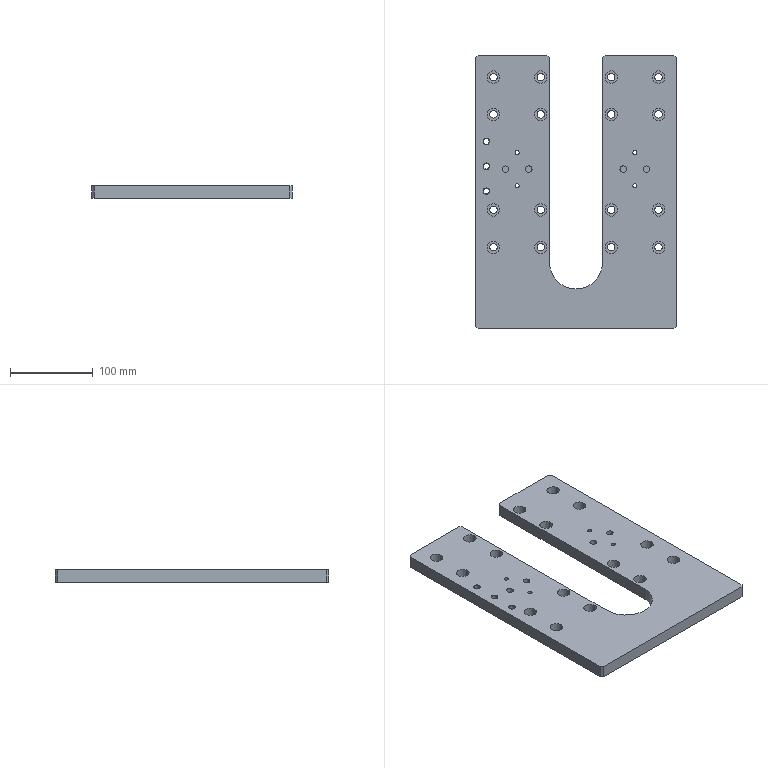Part | SolidWorks | features HoleWzd 4, Chamfer 1, Extrusion 1 | 1 solid | 128 faces | box 242 x 330 x 15 mm | volume 894484 mm3 | cylinder 87 | plane 35 | cone 6 | commonest cylinder face diameters 9 x32 15 x32 5 x8 8 x8 6.8 x6 64 x1